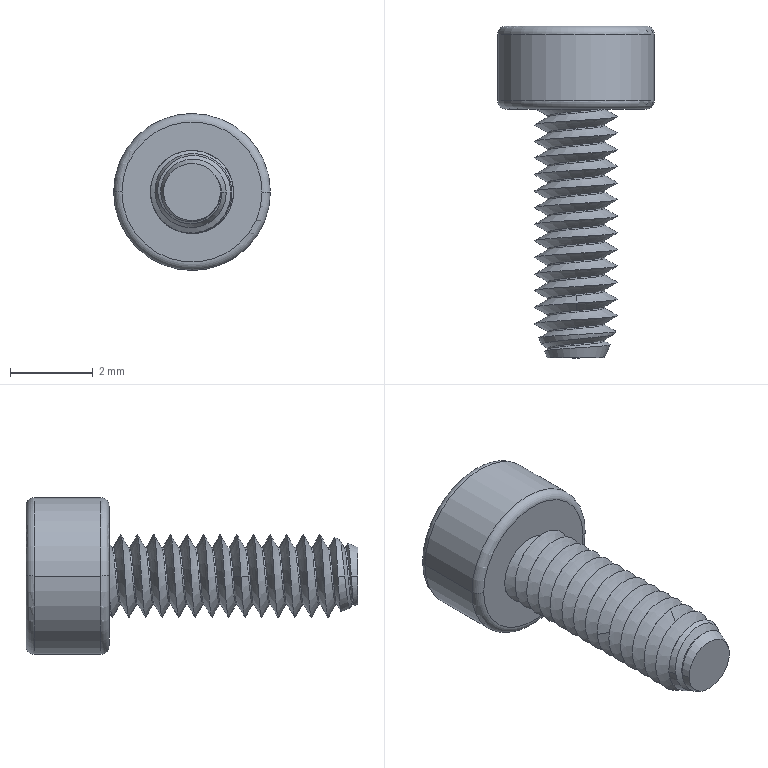Part | SolidWorks | features BaseBody 1 | 1 solid | 70 faces | box 3.78 x 8 x 3.78 mm | volume 33.075 mm3 | cylinder 39 | plane 10 | spline 10 | cone 7 | torus 4 | commonest cylinder face diameters 1.376 x31 0.4 x6 3.78 x2